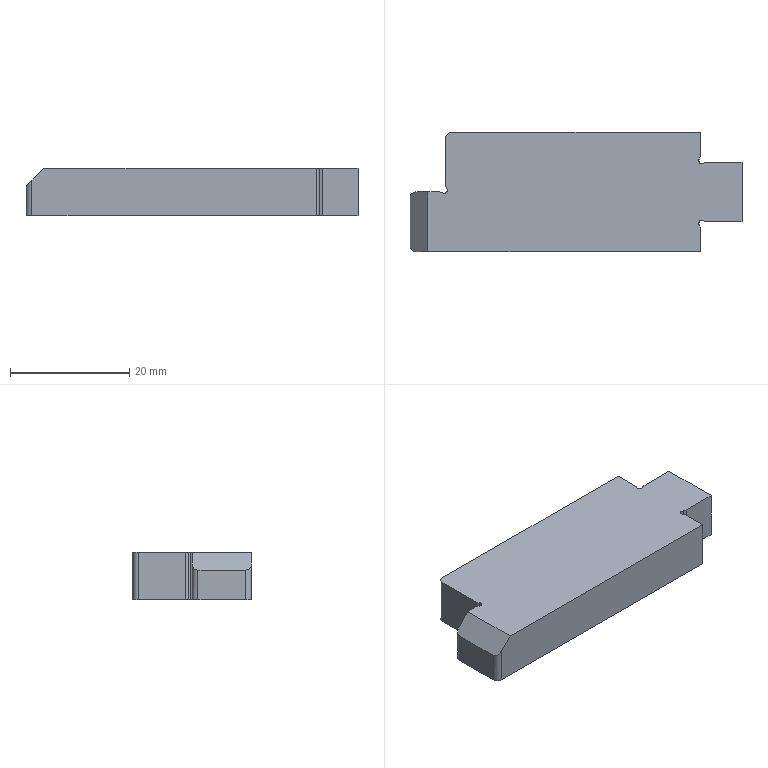Part | SolidWorks | features Chamfer 1, Fillet 1, FlatPattern 1, ICE 1, SMBaseFlange 1, SheetMetal 1 | 1 solid | 26 faces | box 55.7 x 20 x 8 mm | volume 7815 mm3 | cylinder 13 | plane 13 | commonest cylinder face diameters 2 x9 1 x4
STEP:
#1=CARTESIAN_POINT('',(1461.75,307.95,-8.));
#2=VERTEX_POINT('',#1);
#3=CARTESIAN_POINT('',(1461.667,308.226,-8.));
#4=VERTEX_POINT('',#3);
#5=CARTESIAN_POINT('',(1461.25,307.95,-8.));
#6=DIRECTION('',(0.,0.,1.));
#7=DIRECTION('',(1.,0.,0.));
#8=AXIS2_PLACEMENT_3D('',#5,#6,#7);
#9=CIRCLE('',#8,0.5);
#10=EDGE_CURVE('',#2,#4,#9,.T.);
#11=ORIENTED_EDGE('',*,*,#10,.F.);
#12=CARTESIAN_POINT('',(1461.75,307.95,0.));
#13=VERTEX_POINT('',#12);
#14=CARTESIAN_POINT('',(1461.75,307.95,-8.));
#15=DIRECTION('',(0.,0.,1.));
#16=VECTOR('',#15,1000.);
#17=LINE('',#14,#16);
#18=EDGE_CURVE('',#2,#13,#17,.T.);
#19=ORIENTED_EDGE('',*,*,#18,.T.);
#20=CARTESIAN_POINT('',(1461.667,308.226,0.));
#21=VERTEX_POINT('',#20);
#22=CARTESIAN_POINT('',(1461.25,307.95,0.));
#23=DIRECTION('',(0.,0.,1.));
#24=DIRECTION('',(1.,0.,0.));
#25=AXIS2_PLACEMENT_3D('',#22,#23,#24);
#26=CIRCLE('',#25,0.5);
#27=EDGE_CURVE('',#13,#21,#26,.T.);
#28=ORIENTED_EDGE('',*,*,#27,.T.);
#29=CARTESIAN_POINT('',(1461.667,308.226,-8.));
#30=DIRECTION('',(0.,0.,-1.));
#31=VECTOR('',#30,1000.);
#32=LINE('',#29,#31);
#33=EDGE_CURVE('',#21,#4,#32,.T.);
#34=ORIENTED_EDGE('',*,*,#33,.T.);
#35=EDGE_LOOP('',(#11,#19,#28,#34));
#36=FACE_OUTER_BOUND('',#35,.T.);
#37=CARTESIAN_POINT('',(1461.25,307.95,-8.));
#38=DIRECTION('',(0.,0.,1.));
#39=DIRECTION('',(1.,0.,0.));
#40=AXIS2_PLACEMENT_3D('',#37,#38,#39);
#41=CYLINDRICAL_SURFACE('',#40,0.5);
#42=ADVANCED_FACE('',(#36),#41,.F.);
#43=CARTESIAN_POINT('',(1456.5,307.7,-8.));
#44=VERTEX_POINT('',#43);
#45=CARTESIAN_POINT('',(1456.5,307.7,-2.));
#46=VERTEX_POINT('',#45);
#47=CARTESIAN_POINT('',(1456.5,307.7,-8.));
#48=DIRECTION('',(0.,0.,1.));
#49=VECTOR('',#48,1000.);
#50=LINE('',#47,#49);
#51=EDGE_CURVE('',#44,#46,#50,.T.);
#52=ORIENTED_EDGE('',*,*,#51,.T.);
#53=CARTESIAN_POINT('',(1458.5,307.7,0.));
#54=VERTEX_POINT('',#53);
#55=CARTESIAN_POINT('',(1456.,307.7,-2.5));
#56=DIRECTION('',(0.7071,0.,0.7071));
#57=VECTOR('',#56,1000.);
#58=LINE('',#55,#57);
#59=EDGE_CURVE('',#46,#54,#58,.T.);
#60=ORIENTED_EDGE('',*,*,#59,.T.);
#61=CARTESIAN_POINT('',(1460.421,307.7,0.));
#62=VERTEX_POINT('',#61);
#63=CARTESIAN_POINT('',(1461.5,307.7,0.));
#64=DIRECTION('',(-1.,0.,0.));
#65=VECTOR('',#64,1000.);
#66=LINE('',#63,#65);
#67=EDGE_CURVE('',#62,#54,#66,.T.);
#68=ORIENTED_EDGE('',*,*,#67,.F.);
#69=CARTESIAN_POINT('',(1460.421,307.7,-8.));
#70=VERTEX_POINT('',#69);
#71=CARTESIAN_POINT('',(1460.421,307.7,-8.));
#72=DIRECTION('',(0.,0.,-1.));
#73=VECTOR('',#72,1000.);
#74=LINE('',#71,#73);
#75=EDGE_CURVE('',#62,#70,#74,.T.);
#76=ORIENTED_EDGE('',*,*,#75,.T.);
#77=CARTESIAN_POINT('',(1461.5,307.7,-8.));
#78=DIRECTION('',(-1.,0.,0.));
#79=VECTOR('',#78,1000.);
#80=LINE('',#77,#79);
#81=EDGE_CURVE('',#70,#44,#80,.T.);
#82=ORIENTED_EDGE('',*,*,#81,.T.);
#83=EDGE_LOOP('',(#52,#60,#68,#76,#82));
#84=FACE_OUTER_BOUND('',#83,.T.);
#85=CARTESIAN_POINT('',(1461.5,307.7,-8.));
#86=DIRECTION('',(0.,1.,0.));
#87=DIRECTION('',(0.,0.,1.));
#88=AXIS2_PLACEMENT_3D('',#85,#86,#87);
#89=PLANE('',#88);
#90=ADVANCED_FACE('',(#84),#89,.T.);
#91=CARTESIAN_POINT('',(1461.5,316.7,0.));
#92=VERTEX_POINT('',#91);
#93=CARTESIAN_POINT('',(1461.5,308.779,0.));
#94=VERTEX_POINT('',#93);
#95=CARTESIAN_POINT('',(1461.5,317.7,0.));
#96=DIRECTION('',(0.,-1.,0.));
#97=VECTOR('',#96,1000.);
#98=LINE('',#95,#97);
#99=EDGE_CURVE('',#92,#94,#98,.T.);
#100=ORIENTED_EDGE('',*,*,#99,.F.);
#101=CARTESIAN_POINT('',(1461.5,316.7,-8.));
#102=VERTEX_POINT('',#101);
#103=CARTESIAN_POINT('',(1461.5,316.7,-8.));
#104=DIRECTION('',(0.,0.,-1.));
#105=VECTOR('',#104,1000.);
#106=LINE('',#103,#105);
#107=EDGE_CURVE('',#92,#102,#106,.T.);
#108=ORIENTED_EDGE('',*,*,#107,.T.);
#109=CARTESIAN_POINT('',(1461.5,308.779,-8.));
#110=VERTEX_POINT('',#109);
#111=CARTESIAN_POINT('',(1461.5,317.7,-8.));
#112=DIRECTION('',(0.,-1.,0.));
#113=VECTOR('',#112,1000.);
#114=LINE('',#111,#113);
#115=EDGE_CURVE('',#102,#110,#114,.T.);
#116=ORIENTED_EDGE('',*,*,#115,.T.);
#117=CARTESIAN_POINT('',(1461.5,308.779,-8.));
#118=DIRECTION('',(0.,0.,1.));
#119=VECTOR('',#118,1000.);
#120=LINE('',#117,#119);
#121=EDGE_CURVE('',#110,#94,#120,.T.);
#122=ORIENTED_EDGE('',*,*,#121,.T.);
#123=EDGE_LOOP('',(#100,#108,#116,#122));
#124=FACE_OUTER_BOUND('',#123,.T.);
#125=CARTESIAN_POINT('',(1461.5,317.7,-8.));
#126=DIRECTION('',(-1.,0.,0.));
#127=DIRECTION('',(0.,0.,1.));
#128=AXIS2_PLACEMENT_3D('',#125,#126,#127);
#129=PLANE('',#128);
#130=ADVANCED_FACE('',(#124),#129,.T.);
#131=CARTESIAN_POINT('',(1504.2,313.779,0.));
#132=VERTEX_POINT('',#131);
#133=CARTESIAN_POINT('',(1504.2,317.7,0.));
#134=VERTEX_POINT('',#133);
#135=CARTESIAN_POINT('',(1504.2,312.7,0.));
#136=DIRECTION('',(0.,1.,0.));
#137=VECTOR('',#136,1000.);
#138=LINE('',#135,#137);
#139=EDGE_CURVE('',#132,#134,#138,.T.);
#140=ORIENTED_EDGE('',*,*,#139,.F.);
#141=CARTESIAN_POINT('',(1504.2,313.779,-8.));
#142=VERTEX_POINT('',#141);
#143=CARTESIAN_POINT('',(1504.2,313.779,-8.));
#144=DIRECTION('',(0.,0.,-1.));
#145=VECTOR('',#144,1000.);
#146=LINE('',#143,#145);
#147=EDGE_CURVE('',#132,#142,#146,.T.);
#148=ORIENTED_EDGE('',*,*,#147,.T.);
#149=CARTESIAN_POINT('',(1504.2,317.7,-8.));
#150=VERTEX_POINT('',#149);
#151=CARTESIAN_POINT('',(1504.2,312.7,-8.));
#152=DIRECTION('',(0.,1.,0.));
#153=VECTOR('',#152,1000.);
#154=LINE('',#151,#153);
#155=EDGE_CURVE('',#142,#150,#154,.T.);
#156=ORIENTED_EDGE('',*,*,#155,.T.);
#157=CARTESIAN_POINT('',(1504.2,317.7,-8.));
#158=DIRECTION('',(0.,0.,1.));
#159=VECTOR('',#158,1000.);
#160=LINE('',#157,#159);
#161=EDGE_CURVE('',#150,#134,#160,.T.);
#162=ORIENTED_EDGE('',*,*,#161,.T.);
#163=EDGE_LOOP('',(#140,#148,#156,#162));
#164=FACE_OUTER_BOUND('',#163,.T.);
#165=CARTESIAN_POINT('',(1504.2,312.7,-8.));
#166=DIRECTION('',(1.,0.,0.));
#167=DIRECTION('',(0.,0.,-1.));
#168=AXIS2_PLACEMENT_3D('',#165,#166,#167);
#169=PLANE('',#168);
#170=ADVANCED_FACE('',(#164),#169,.T.);
#171=CARTESIAN_POINT('',(1511.2,312.7,-8.));
#172=VERTEX_POINT('',#171);
#173=CARTESIAN_POINT('',(1505.279,312.7,-8.));
#174=VERTEX_POINT('',#173);
#175=CARTESIAN_POINT('',(1511.2,312.7,-8.));
#176=DIRECTION('',(-1.,0.,0.));
#177=VECTOR('',#176,1000.);
#178=LINE('',#175,#177);
#179=EDGE_CURVE('',#172,#174,#178,.T.);
#180=ORIENTED_EDGE('',*,*,#179,.T.);
#181=CARTESIAN_POINT('',(1505.279,312.7,0.));
#182=VERTEX_POINT('',#181);
#183=CARTESIAN_POINT('',(1505.279,312.7,-8.));
#184=DIRECTION('',(0.,0.,1.));
#185=VECTOR('',#184,1000.);
#186=LINE('',#183,#185);
#187=EDGE_CURVE('',#174,#182,#186,.T.);
#188=ORIENTED_EDGE('',*,*,#187,.T.);
#189=CARTESIAN_POINT('',(1511.2,312.7,0.));
#190=VERTEX_POINT('',#189);
#191=CARTESIAN_POINT('',(1511.2,312.7,0.));
#192=DIRECTION('',(-1.,0.,0.));
#193=VECTOR('',#192,1000.);
#194=LINE('',#191,#193);
#195=EDGE_CURVE('',#190,#182,#194,.T.);
#196=ORIENTED_EDGE('',*,*,#195,.F.);
#197=CARTESIAN_POINT('',(1511.2,312.7,-8.));
#198=DIRECTION('',(0.,0.,1.));
#199=VECTOR('',#198,1000.);
#200=LINE('',#197,#199);
#201=EDGE_CURVE('',#172,#190,#200,.T.);
#202=ORIENTED_EDGE('',*,*,#201,.F.);
#203=EDGE_LOOP('',(#180,#188,#196,#202));
#204=FACE_OUTER_BOUND('',#203,.T.);
#205=CARTESIAN_POINT('',(1511.2,312.7,-8.));
#206=DIRECTION('',(0.,1.,0.));
#207=DIRECTION('',(0.,0.,1.));
#208=AXIS2_PLACEMENT_3D('',#205,#206,#207);
#209=PLANE('',#208);
#210=ADVANCED_FACE('',(#204),#209,.T.);
#211=CARTESIAN_POINT('',(1505.279,302.7,0.));
#212=VERTEX_POINT('',#211);
#213=CARTESIAN_POINT('',(1511.2,302.7,0.));
#214=VERTEX_POINT('',#213);
#215=CARTESIAN_POINT('',(1504.2,302.7,0.));
#216=DIRECTION('',(1.,0.,0.));
#217=VECTOR('',#216,1000.);
#218=LINE('',#215,#217);
#219=EDGE_CURVE('',#212,#214,#218,.T.);
#220=ORIENTED_EDGE('',*,*,#219,.F.);
#221=CARTESIAN_POINT('',(1505.279,302.7,-8.));
#222=VERTEX_POINT('',#221);
#223=CARTESIAN_POINT('',(1505.279,302.7,-8.));
#224=DIRECTION('',(0.,0.,-1.));
#225=VECTOR('',#224,1000.);
#226=LINE('',#223,#225);
#227=EDGE_CURVE('',#212,#222,#226,.T.);
#228=ORIENTED_EDGE('',*,*,#227,.T.);
#229=CARTESIAN_POINT('',(1511.2,302.7,-8.));
#230=VERTEX_POINT('',#229);
#231=CARTESIAN_POINT('',(1504.2,302.7,-8.));
#232=DIRECTION('',(1.,0.,0.));
#233=VECTOR('',#232,1000.);
#234=LINE('',#231,#233);
#235=EDGE_CURVE('',#222,#230,#234,.T.);
#236=ORIENTED_EDGE('',*,*,#235,.T.);
#237=CARTESIAN_POINT('',(1511.2,302.7,-8.));
#238=DIRECTION('',(0.,0.,1.));
#239=VECTOR('',#238,1000.);
#240=LINE('',#237,#239);
#241=EDGE_CURVE('',#230,#214,#240,.T.);
#242=ORIENTED_EDGE('',*,*,#241,.T.);
#243=EDGE_LOOP('',(#220,#228,#236,#242));
#244=FACE_OUTER_BOUND('',#243,.T.);
#245=CARTESIAN_POINT('',(1504.2,302.7,-8.));
#246=DIRECTION('',(0.,-1.,0.));
#247=DIRECTION('',(0.,0.,-1.));
#248=AXIS2_PLACEMENT_3D('',#245,#246,#247);
#249=PLANE('',#248);
#250=ADVANCED_FACE('',(#244),#249,.T.);
#251=CARTESIAN_POINT('',(1504.2,297.7,-8.));
#252=VERTEX_POINT('',#251);
#253=CARTESIAN_POINT('',(1504.2,301.621,-8.));
#254=VERTEX_POINT('',#253);
#255=CARTESIAN_POINT('',(1504.2,297.7,-8.));
#256=DIRECTION('',(0.,1.,0.));
#257=VECTOR('',#256,1000.);
#258=LINE('',#255,#257);
#259=EDGE_CURVE('',#252,#254,#258,.T.);
#260=ORIENTED_EDGE('',*,*,#259,.T.);
#261=CARTESIAN_POINT('',(1504.2,301.621,0.));
#262=VERTEX_POINT('',#261);
#263=CARTESIAN_POINT('',(1504.2,301.621,-8.));
#264=DIRECTION('',(0.,0.,1.));
#265=VECTOR('',#264,1000.);
#266=LINE('',#263,#265);
#267=EDGE_CURVE('',#254,#262,#266,.T.);
#268=ORIENTED_EDGE('',*,*,#267,.T.);
#269=CARTESIAN_POINT('',(1504.2,297.7,0.));
#270=VERTEX_POINT('',#269);
#271=CARTESIAN_POINT('',(1504.2,297.7,0.));
#272=DIRECTION('',(0.,1.,0.));
#273=VECTOR('',#272,1000.);
#274=LINE('',#271,#273);
#275=EDGE_CURVE('',#270,#262,#274,.T.);
#276=ORIENTED_EDGE('',*,*,#275,.F.);
#277=CARTESIAN_POINT('',(1504.2,297.7,-8.));
#278=DIRECTION('',(0.,0.,1.));
#279=VECTOR('',#278,1000.);
#280=LINE('',#277,#279);
#281=EDGE_CURVE('',#252,#270,#280,.T.);
#282=ORIENTED_EDGE('',*,*,#281,.F.);
#283=EDGE_LOOP('',(#260,#268,#276,#282));
#284=FACE_OUTER_BOUND('',#283,.T.);
#285=CARTESIAN_POINT('',(1504.2,297.7,-8.));
#286=DIRECTION('',(1.,0.,0.));
#287=DIRECTION('',(0.,0.,-1.));
#288=AXIS2_PLACEMENT_3D('',#285,#286,#287);
#289=PLANE('',#288);
#290=ADVANCED_FACE('',(#284),#289,.T.);
#291=CARTESIAN_POINT('',(1455.5,306.7,-8.));
#292=VERTEX_POINT('',#291);
#293=CARTESIAN_POINT('',(1455.5,298.7,-8.));
#294=VERTEX_POINT('',#293);
#295=CARTESIAN_POINT('',(1455.5,307.7,-8.));
#296=DIRECTION('',(0.,-1.,0.));
#297=VECTOR('',#296,1000.);
#298=LINE('',#295,#297);
#299=EDGE_CURVE('',#292,#294,#298,.T.);
#300=ORIENTED_EDGE('',*,*,#299,.F.);
#301=CARTESIAN_POINT('',(1456.5,306.7,-8.));
#302=DIRECTION('',(0.,0.,-1.));
#303=DIRECTION('',(1.,0.,0.));
#304=AXIS2_PLACEMENT_3D('',#301,#302,#303);
#305=CIRCLE('',#304,1.);
#306=EDGE_CURVE('',#292,#44,#305,.T.);
#307=ORIENTED_EDGE('',*,*,#306,.T.);
#308=ORIENTED_EDGE('',*,*,#81,.F.);
#309=CARTESIAN_POINT('',(1460.974,307.533,-8.));
#310=VERTEX_POINT('',#309);
#311=CARTESIAN_POINT('',(1460.421,306.7,-8.));
#312=DIRECTION('',(0.,0.,-1.));
#313=DIRECTION('',(1.,0.,0.));
#314=AXIS2_PLACEMENT_3D('',#311,#312,#313);
#315=CIRCLE('',#314,1.);
#316=EDGE_CURVE('',#70,#310,#315,.T.);
#317=ORIENTED_EDGE('',*,*,#316,.T.);
#318=CARTESIAN_POINT('',(1461.25,307.95,-8.));
#319=DIRECTION('',(0.,0.,1.));
#320=DIRECTION('',(1.,0.,0.));
#321=AXIS2_PLACEMENT_3D('',#318,#319,#320);
#322=CIRCLE('',#321,0.5);
#323=EDGE_CURVE('',#310,#2,#322,.T.);
#324=ORIENTED_EDGE('',*,*,#323,.T.);
#325=ORIENTED_EDGE('',*,*,#10,.T.);
#326=CARTESIAN_POINT('',(1462.5,308.779,-8.));
#327=DIRECTION('',(0.,0.,-1.));
#328=DIRECTION('',(1.,0.,0.));
#329=AXIS2_PLACEMENT_3D('',#326,#327,#328);
#330=CIRCLE('',#329,1.);
#331=EDGE_CURVE('',#4,#110,#330,.T.);
#332=ORIENTED_EDGE('',*,*,#331,.T.);
#333=ORIENTED_EDGE('',*,*,#115,.F.);
#334=CARTESIAN_POINT('',(1462.5,317.7,-8.));
#335=VERTEX_POINT('',#334);
#336=CARTESIAN_POINT('',(1462.5,316.7,-8.));
#337=DIRECTION('',(0.,0.,-1.));
#338=DIRECTION('',(1.,0.,0.));
#339=AXIS2_PLACEMENT_3D('',#336,#337,#338);
#340=CIRCLE('',#339,1.);
#341=EDGE_CURVE('',#102,#335,#340,.T.);
#342=ORIENTED_EDGE('',*,*,#341,.T.);
#343=CARTESIAN_POINT('',(1504.2,317.7,-8.));
#344=DIRECTION('',(-1.,0.,0.));
#345=VECTOR('',#344,1000.);
#346=LINE('',#343,#345);
#347=EDGE_CURVE('',#150,#335,#346,.T.);
#348=ORIENTED_EDGE('',*,*,#347,.F.);
#349=ORIENTED_EDGE('',*,*,#155,.F.);
#350=CARTESIAN_POINT('',(1504.033,313.226,-8.));
#351=VERTEX_POINT('',#350);
#352=CARTESIAN_POINT('',(1503.2,313.779,-8.));
#353=DIRECTION('',(0.,0.,-1.));
#354=DIRECTION('',(1.,0.,0.));
#355=AXIS2_PLACEMENT_3D('',#352,#353,#354);
#356=CIRCLE('',#355,1.);
#357=EDGE_CURVE('',#142,#351,#356,.T.);
#358=ORIENTED_EDGE('',*,*,#357,.T.);
#359=CARTESIAN_POINT('',(1504.726,312.533,-8.));
#360=VERTEX_POINT('',#359);
#361=CARTESIAN_POINT('',(1504.45,312.95,-8.));
#362=DIRECTION('',(0.,0.,1.));
#363=DIRECTION('',(1.,0.,0.));
#364=AXIS2_PLACEMENT_3D('',#361,#362,#363);
#365=CIRCLE('',#364,0.5);
#366=EDGE_CURVE('',#351,#360,#365,.T.);
#367=ORIENTED_EDGE('',*,*,#366,.T.);
#368=CARTESIAN_POINT('',(1505.279,311.7,-8.));
#369=DIRECTION('',(0.,0.,-1.));
#370=DIRECTION('',(1.,0.,0.));
#371=AXIS2_PLACEMENT_3D('',#368,#369,#370);
#372=CIRCLE('',#371,1.);
#373=EDGE_CURVE('',#360,#174,#372,.T.);
#374=ORIENTED_EDGE('',*,*,#373,.T.);
#375=ORIENTED_EDGE('',*,*,#179,.F.);
#376=CARTESIAN_POINT('',(1511.2,302.7,-8.));
#377=DIRECTION('',(0.,1.,0.));
#378=VECTOR('',#377,1000.);
#379=LINE('',#376,#378);
#380=EDGE_CURVE('',#230,#172,#379,.T.);
#381=ORIENTED_EDGE('',*,*,#380,.F.);
#382=ORIENTED_EDGE('',*,*,#235,.F.);
#383=CARTESIAN_POINT('',(1504.726,302.867,-8.));
#384=VERTEX_POINT('',#383);
#385=CARTESIAN_POINT('',(1505.279,303.7,-8.));
#386=DIRECTION('',(0.,0.,-1.));
#387=DIRECTION('',(1.,0.,0.));
#388=AXIS2_PLACEMENT_3D('',#385,#386,#387);
#389=CIRCLE('',#388,1.);
#390=EDGE_CURVE('',#222,#384,#389,.T.);
#391=ORIENTED_EDGE('',*,*,#390,.T.);
#392=CARTESIAN_POINT('',(1504.033,302.174,-8.));
#393=VERTEX_POINT('',#392);
#394=CARTESIAN_POINT('',(1504.45,302.45,-8.));
#395=DIRECTION('',(0.,0.,1.));
#396=DIRECTION('',(1.,0.,0.));
#397=AXIS2_PLACEMENT_3D('',#394,#395,#396);
#398=CIRCLE('',#397,0.5);
#399=EDGE_CURVE('',#384,#393,#398,.T.);
#400=ORIENTED_EDGE('',*,*,#399,.T.);
#401=CARTESIAN_POINT('',(1503.2,301.621,-8.));
#402=DIRECTION('',(0.,0.,-1.));
#403=DIRECTION('',(1.,0.,0.));
#404=AXIS2_PLACEMENT_3D('',#401,#402,#403);
#405=CIRCLE('',#404,1.);
#406=EDGE_CURVE('',#393,#254,#405,.T.);
#407=ORIENTED_EDGE('',*,*,#406,.T.);
#408=ORIENTED_EDGE('',*,*,#259,.F.);
#409=CARTESIAN_POINT('',(1456.5,297.7,-8.));
#410=VERTEX_POINT('',#409);
#411=CARTESIAN_POINT('',(1455.5,297.7,-8.));
#412=DIRECTION('',(1.,0.,0.));
#413=VECTOR('',#412,1000.);
#414=LINE('',#411,#413);
#415=EDGE_CURVE('',#410,#252,#414,.T.);
#416=ORIENTED_EDGE('',*,*,#415,.F.);
#417=CARTESIAN_POINT('',(1456.5,298.7,-8.));
#418=DIRECTION('',(0.,0.,-1.));
#419=DIRECTION('',(1.,0.,0.));
#420=AXIS2_PLACEMENT_3D('',#417,#418,#419);
#421=CIRCLE('',#420,1.);
#422=EDGE_CURVE('',#410,#294,#421,.T.);
#423=ORIENTED_EDGE('',*,*,#422,.T.);
#424=EDGE_LOOP('',(#300,#307,#308,#317,#324,#325,#332,#333,#342,#348,#349,#358,#367,#374,#375,#381,#382,#391,#400,#407,#408,#416,#423));
#425=FACE_OUTER_BOUND('',#424,.T.);
#426=CARTESIAN_POINT('',(0.,0.,-8.));
#427=DIRECTION('',(0.,0.,1.));
#428=DIRECTION('',(1.,0.,0.));
#429=AXIS2_PLACEMENT_3D('',#426,#427,#428);
#430=PLANE('',#429);
#431=ADVANCED_FACE('',(#425),#430,.F.);
#432=ORIENTED_EDGE('',*,*,#67,.T.);
#433=CARTESIAN_POINT('',(1458.5,297.7,0.));
#434=VERTEX_POINT('',#433);
#435=CARTESIAN_POINT('',(1458.5,0.,0.));
#436=DIRECTION('',(0.,-1.,0.));
#437=VECTOR('',#436,1000.);
#438=LINE('',#435,#437);
#439=EDGE_CURVE('',#54,#434,#438,.T.);
#440=ORIENTED_EDGE('',*,*,#439,.T.);
#441=CARTESIAN_POINT('',(1455.5,297.7,0.));
#442=DIRECTION('',(1.,0.,0.));
#443=VECTOR('',#442,1000.);
#444=LINE('',#441,#443);
#445=EDGE_CURVE('',#434,#270,#444,.T.);
#446=ORIENTED_EDGE('',*,*,#445,.T.);
#447=ORIENTED_EDGE('',*,*,#275,.T.);
#448=CARTESIAN_POINT('',(1504.033,302.174,0.));
#449=VERTEX_POINT('',#448);
#450=CARTESIAN_POINT('',(1503.2,301.621,0.));
#451=DIRECTION('',(0.,0.,1.));
#452=DIRECTION('',(1.,0.,0.));
#453=AXIS2_PLACEMENT_3D('',#450,#451,#452);
#454=CIRCLE('',#453,1.);
#455=EDGE_CURVE('',#262,#449,#454,.T.);
#456=ORIENTED_EDGE('',*,*,#455,.T.);
#457=CARTESIAN_POINT('',(1504.726,302.867,0.));
#458=VERTEX_POINT('',#457);
#459=CARTESIAN_POINT('',(1504.45,302.45,0.));
#460=DIRECTION('',(0.,0.,1.));
#461=DIRECTION('',(1.,0.,0.));
#462=AXIS2_PLACEMENT_3D('',#459,#460,#461);
#463=CIRCLE('',#462,0.5);
#464=EDGE_CURVE('',#458,#449,#463,.T.);
#465=ORIENTED_EDGE('',*,*,#464,.F.);
#466=CARTESIAN_POINT('',(1505.279,303.7,0.));
#467=DIRECTION('',(0.,0.,1.));
#468=DIRECTION('',(1.,0.,0.));
#469=AXIS2_PLACEMENT_3D('',#466,#467,#468);
#470=CIRCLE('',#469,1.);
#471=EDGE_CURVE('',#458,#212,#470,.T.);
#472=ORIENTED_EDGE('',*,*,#471,.T.);
#473=ORIENTED_EDGE('',*,*,#219,.T.);
#474=CARTESIAN_POINT('',(1511.2,302.7,0.));
#475=DIRECTION('',(0.,1.,0.));
#476=VECTOR('',#475,1000.);
#477=LINE('',#474,#476);
#478=EDGE_CURVE('',#214,#190,#477,.T.);
#479=ORIENTED_EDGE('',*,*,#478,.T.);
#480=ORIENTED_EDGE('',*,*,#195,.T.);
#481=CARTESIAN_POINT('',(1504.726,312.533,0.));
#482=VERTEX_POINT('',#481);
#483=CARTESIAN_POINT('',(1505.279,311.7,0.));
#484=DIRECTION('',(0.,0.,1.));
#485=DIRECTION('',(1.,0.,0.));
#486=AXIS2_PLACEMENT_3D('',#483,#484,#485);
#487=CIRCLE('',#486,1.);
#488=EDGE_CURVE('',#182,#482,#487,.T.);
#489=ORIENTED_EDGE('',*,*,#488,.T.);
#490=CARTESIAN_POINT('',(1504.033,313.226,0.));
#491=VERTEX_POINT('',#490);
#492=CARTESIAN_POINT('',(1504.45,312.95,0.));
#493=DIRECTION('',(0.,0.,1.));
#494=DIRECTION('',(1.,0.,0.));
#495=AXIS2_PLACEMENT_3D('',#492,#493,#494);
#496=CIRCLE('',#495,0.5);
#497=EDGE_CURVE('',#491,#482,#496,.T.);
#498=ORIENTED_EDGE('',*,*,#497,.F.);
#499=CARTESIAN_POINT('',(1503.2,313.779,0.));
#500=DIRECTION('',(0.,0.,1.));
#501=DIRECTION('',(1.,0.,0.));
#502=AXIS2_PLACEMENT_3D('',#499,#500,#501);
#503=CIRCLE('',#502,1.);
#504=EDGE_CURVE('',#491,#132,#503,.T.);
#505=ORIENTED_EDGE('',*,*,#504,.T.);
#506=ORIENTED_EDGE('',*,*,#139,.T.);
#507=CARTESIAN_POINT('',(1462.5,317.7,0.));
#508=VERTEX_POINT('',#507);
#509=CARTESIAN_POINT('',(1504.2,317.7,0.));
#510=DIRECTION('',(-1.,0.,0.));
#511=VECTOR('',#510,1000.);
#512=LINE('',#509,#511);
#513=EDGE_CURVE('',#134,#508,#512,.T.);
#514=ORIENTED_EDGE('',*,*,#513,.T.);
#515=CARTESIAN_POINT('',(1462.5,316.7,0.));
#516=DIRECTION('',(0.,0.,1.));
#517=DIRECTION('',(1.,0.,0.));
#518=AXIS2_PLACEMENT_3D('',#515,#516,#517);
#519=CIRCLE('',#518,1.);
#520=EDGE_CURVE('',#508,#92,#519,.T.);
#521=ORIENTED_EDGE('',*,*,#520,.T.);
#522=ORIENTED_EDGE('',*,*,#99,.T.);
#523=CARTESIAN_POINT('',(1462.5,308.779,0.));
#524=DIRECTION('',(0.,0.,1.));
#525=DIRECTION('',(1.,0.,0.));
#526=AXIS2_PLACEMENT_3D('',#523,#524,#525);
#527=CIRCLE('',#526,1.);
#528=EDGE_CURVE('',#94,#21,#527,.T.);
#529=ORIENTED_EDGE('',*,*,#528,.T.);
#530=ORIENTED_EDGE('',*,*,#27,.F.);
#531=CARTESIAN_POINT('',(1460.974,307.533,0.));
#532=VERTEX_POINT('',#531);
#533=CARTESIAN_POINT('',(1461.25,307.95,0.));
#534=DIRECTION('',(0.,0.,1.));
#535=DIRECTION('',(1.,0.,0.));
#536=AXIS2_PLACEMENT_3D('',#533,#534,#535);
#537=CIRCLE('',#536,0.5);
#538=EDGE_CURVE('',#532,#13,#537,.T.);
#539=ORIENTED_EDGE('',*,*,#538,.F.);
#540=CARTESIAN_POINT('',(1460.421,306.7,0.));
#541=DIRECTION('',(0.,0.,1.));
#542=DIRECTION('',(1.,0.,0.));
#543=AXIS2_PLACEMENT_3D('',#540,#541,#542);
#544=CIRCLE('',#543,1.);
#545=EDGE_CURVE('',#532,#62,#544,.T.);
#546=ORIENTED_EDGE('',*,*,#545,.T.);
#547=EDGE_LOOP('',(#432,#440,#446,#447,#456,#465,#472,#473,#479,#480,#489,#498,#505,#506,#514,#521,#522,#529,#530,#539,#546));
#548=FACE_OUTER_BOUND('',#547,.T.);
#549=CARTESIAN_POINT('',(0.,0.,0.));
#550=DIRECTION('',(0.,0.,1.));
#551=DIRECTION('',(1.,0.,0.));
#552=AXIS2_PLACEMENT_3D('',#549,#550,#551);
#553=PLANE('',#552);
#554=ADVANCED_FACE('',(#548),#553,.T.);
#555=ORIENTED_EDGE('',*,*,#347,.T.);
#556=CARTESIAN_POINT('',(1462.5,317.7,-8.));
#557=DIRECTION('',(0.,0.,1.));
#558=VECTOR('',#557,1000.);
#559=LINE('',#556,#558);
#560=EDGE_CURVE('',#335,#508,#559,.T.);
#561=ORIENTED_EDGE('',*,*,#560,.T.);
#562=ORIENTED_EDGE('',*,*,#513,.F.);
#563=ORIENTED_EDGE('',*,*,#161,.F.);
#564=EDGE_LOOP('',(#555,#561,#562,#563));
#565=FACE_OUTER_BOUND('',#564,.T.);
#566=CARTESIAN_POINT('',(1504.2,317.7,-8.));
#567=DIRECTION('',(0.,1.,0.));
#568=DIRECTION('',(0.,0.,1.));
#569=AXIS2_PLACEMENT_3D('',#566,#567,#568);
#570=PLANE('',#569);
#571=ADVANCED_FACE('',(#565),#570,.T.);
#572=ORIENTED_EDGE('',*,*,#478,.F.);
#573=ORIENTED_EDGE('',*,*,#241,.F.);
#574=ORIENTED_EDGE('',*,*,#380,.T.);
#575=ORIENTED_EDGE('',*,*,#201,.T.);
#576=EDGE_LOOP('',(#572,#573,#574,#575));
#577=FACE_OUTER_BOUND('',#576,.T.);
#578=CARTESIAN_POINT('',(1511.2,302.7,-8.));
#579=DIRECTION('',(1.,0.,0.));
#580=DIRECTION('',(0.,0.,-1.));
#581=AXIS2_PLACEMENT_3D('',#578,#579,#580);
#582=PLANE('',#581);
#583=ADVANCED_FACE('',(#577),#582,.T.);
#584=ORIENTED_EDGE('',*,*,#445,.F.);
#585=CARTESIAN_POINT('',(1456.5,297.7,-2.));
#586=VERTEX_POINT('',#585);
#587=CARTESIAN_POINT('',(1453.,297.7,-5.5));
#588=DIRECTION('',(-0.7071,0.,-0.7071));
#589=VECTOR('',#588,1000.);
#590=LINE('',#587,#589);
#591=EDGE_CURVE('',#434,#586,#590,.T.);
#592=ORIENTED_EDGE('',*,*,#591,.T.);
#593=CARTESIAN_POINT('',(1456.5,297.7,-8.));
#594=DIRECTION('',(0.,0.,-1.));
#595=VECTOR('',#594,1000.);
#596=LINE('',#593,#595);
#597=EDGE_CURVE('',#586,#410,#596,.T.);
#598=ORIENTED_EDGE('',*,*,#597,.T.);
#599=ORIENTED_EDGE('',*,*,#415,.T.);
#600=ORIENTED_EDGE('',*,*,#281,.T.);
#601=EDGE_LOOP('',(#584,#592,#598,#599,#600));
#602=FACE_OUTER_BOUND('',#601,.T.);
#603=CARTESIAN_POINT('',(1455.5,297.7,-8.));
#604=DIRECTION('',(0.,-1.,0.));
#605=DIRECTION('',(0.,0.,-1.));
#606=AXIS2_PLACEMENT_3D('',#603,#604,#605);
#607=PLANE('',#606);
#608=ADVANCED_FACE('',(#602),#607,.T.);
#609=CARTESIAN_POINT('',(1455.5,298.7,-3.));
#610=VERTEX_POINT('',#609);
#611=CARTESIAN_POINT('',(1455.5,298.7,-8.));
#612=DIRECTION('',(0.,0.,1.));
#613=VECTOR('',#612,1000.);
#614=LINE('',#611,#613);
#615=EDGE_CURVE('',#294,#610,#614,.T.);
#616=ORIENTED_EDGE('',*,*,#615,.T.);
#617=CARTESIAN_POINT('',(1455.5,306.7,-3.));
#618=VERTEX_POINT('',#617);
#619=CARTESIAN_POINT('',(1455.5,307.7,-3.));
#620=DIRECTION('',(0.,1.,0.));
#621=VECTOR('',#620,1000.);
#622=LINE('',#619,#621);
#623=EDGE_CURVE('',#610,#618,#622,.T.);
#624=ORIENTED_EDGE('',*,*,#623,.T.);
#625=CARTESIAN_POINT('',(1455.5,306.7,-8.));
#626=DIRECTION('',(0.,0.,-1.));
#627=VECTOR('',#626,1000.);
#628=LINE('',#625,#627);
#629=EDGE_CURVE('',#618,#292,#628,.T.);
#630=ORIENTED_EDGE('',*,*,#629,.T.);
#631=ORIENTED_EDGE('',*,*,#299,.T.);
#632=EDGE_LOOP('',(#616,#624,#630,#631));
#633=FACE_OUTER_BOUND('',#632,.T.);
#634=CARTESIAN_POINT('',(1455.5,307.7,-8.));
#635=DIRECTION('',(-1.,0.,0.));
#636=DIRECTION('',(0.,0.,1.));
#637=AXIS2_PLACEMENT_3D('',#634,#635,#636);
#638=PLANE('',#637);
#639=ADVANCED_FACE('',(#633),#638,.T.);
#640=ORIENTED_EDGE('',*,*,#497,.T.);
#641=CARTESIAN_POINT('',(1504.726,312.533,-8.));
#642=DIRECTION('',(0.,0.,-1.));
#643=VECTOR('',#642,1000.);
#644=LINE('',#641,#643);
#645=EDGE_CURVE('',#482,#360,#644,.T.);
#646=ORIENTED_EDGE('',*,*,#645,.T.);
#647=ORIENTED_EDGE('',*,*,#366,.F.);
#648=CARTESIAN_POINT('',(1504.033,313.226,-8.));
#649=DIRECTION('',(0.,0.,1.));
#650=VECTOR('',#649,1000.);
#651=LINE('',#648,#650);
#652=EDGE_CURVE('',#351,#491,#651,.T.);
#653=ORIENTED_EDGE('',*,*,#652,.T.);
#654=EDGE_LOOP('',(#640,#646,#647,#653));
#655=FACE_OUTER_BOUND('',#654,.T.);
#656=CARTESIAN_POINT('',(1504.45,312.95,-8.));
#657=DIRECTION('',(0.,0.,1.));
#658=DIRECTION('',(1.,0.,0.));
#659=AXIS2_PLACEMENT_3D('',#656,#657,#658);
#660=CYLINDRICAL_SURFACE('',#659,0.5);
#661=ADVANCED_FACE('',(#655),#660,.F.);
#662=ORIENTED_EDGE('',*,*,#18,.F.);
#663=ORIENTED_EDGE('',*,*,#323,.F.);
#664=CARTESIAN_POINT('',(1460.974,307.533,-8.));
#665=DIRECTION('',(0.,0.,1.));
#666=VECTOR('',#665,1000.);
#667=LINE('',#664,#666);
#668=EDGE_CURVE('',#310,#532,#667,.T.);
#669=ORIENTED_EDGE('',*,*,#668,.T.);
#670=ORIENTED_EDGE('',*,*,#538,.T.);
#671=EDGE_LOOP('',(#662,#663,#669,#670));
#672=FACE_OUTER_BOUND('',#671,.T.);
#673=CARTESIAN_POINT('',(1461.25,307.95,-8.));
#674=DIRECTION('',(0.,0.,1.));
#675=DIRECTION('',(1.,0.,0.));
#676=AXIS2_PLACEMENT_3D('',#673,#674,#675);
#677=CYLINDRICAL_SURFACE('',#676,0.5);
#678=ADVANCED_FACE('',(#672),#677,.F.);
#679=ORIENTED_EDGE('',*,*,#399,.F.);
#680=CARTESIAN_POINT('',(1504.726,302.867,-8.));
#681=DIRECTION('',(0.,0.,1.));
#682=VECTOR('',#681,1000.);
#683=LINE('',#680,#682);
#684=EDGE_CURVE('',#384,#458,#683,.T.);
#685=ORIENTED_EDGE('',*,*,#684,.T.);
#686=ORIENTED_EDGE('',*,*,#464,.T.);
#687=CARTESIAN_POINT('',(1504.033,302.174,-8.));
#688=DIRECTION('',(0.,0.,-1.));
#689=VECTOR('',#688,1000.);
#690=LINE('',#687,#689);
#691=EDGE_CURVE('',#449,#393,#690,.T.);
#692=ORIENTED_EDGE('',*,*,#691,.T.);
#693=EDGE_LOOP('',(#679,#685,#686,#692));
#694=FACE_OUTER_BOUND('',#693,.T.);
#695=CARTESIAN_POINT('',(1504.45,302.45,-8.));
#696=DIRECTION('',(0.,0.,1.));
#697=DIRECTION('',(1.,0.,0.));
#698=AXIS2_PLACEMENT_3D('',#695,#696,#697);
#699=CYLINDRICAL_SURFACE('',#698,0.5);
#700=ADVANCED_FACE('',(#694),#699,.F.);
#701=ORIENTED_EDGE('',*,*,#629,.F.);
#702=CARTESIAN_POINT('',(1455.5,306.7,-3.));
#703=CARTESIAN_POINT('',(1455.5,307.286,-3.));
#704=CARTESIAN_POINT('',(1455.914,307.7,-2.586));
#705=CARTESIAN_POINT('',(1456.5,307.7,-2.));
#706=(BOUNDED_CURVE()B_SPLINE_CURVE(3,(#702,#703,#704,#705),.UNSPECIFIED.,.F.,.T.)B_SPLINE_CURVE_WITH_KNOTS((4,4),(3.142,4.712),.UNSPECIFIED.)CURVE()GEOMETRIC_REPRESENTATION_ITEM()RATIONAL_B_SPLINE_CURVE((1.,0.8047,0.8047,1.))REPRESENTATION_ITEM(''));
#707=EDGE_CURVE('',#618,#46,#706,.T.);
#708=ORIENTED_EDGE('',*,*,#707,.T.);
#709=ORIENTED_EDGE('',*,*,#51,.F.);
#710=ORIENTED_EDGE('',*,*,#306,.F.);
#711=EDGE_LOOP('',(#701,#708,#709,#710));
#712=FACE_OUTER_BOUND('',#711,.T.);
#713=CARTESIAN_POINT('',(1456.5,306.7,-8.));
#714=DIRECTION('',(0.,0.,1.));
#715=DIRECTION('',(1.,0.,0.));
#716=AXIS2_PLACEMENT_3D('',#713,#714,#715);
#717=CYLINDRICAL_SURFACE('',#716,1.);
#718=ADVANCED_FACE('',(#712),#717,.T.);
#719=ORIENTED_EDGE('',*,*,#597,.F.);
#720=CARTESIAN_POINT('',(1456.5,297.7,-2.));
#721=CARTESIAN_POINT('',(1455.914,297.7,-2.586));
#722=CARTESIAN_POINT('',(1455.5,298.114,-3.));
#723=CARTESIAN_POINT('',(1455.5,298.7,-3.));
#724=(BOUNDED_CURVE()B_SPLINE_CURVE(3,(#720,#721,#722,#723),.UNSPECIFIED.,.F.,.T.)B_SPLINE_CURVE_WITH_KNOTS((4,4),(1.571,3.142),.UNSPECIFIED.)CURVE()GEOMETRIC_REPRESENTATION_ITEM()RATIONAL_B_SPLINE_CURVE((1.,0.8047,0.8047,1.))REPRESENTATION_ITEM(''));
#725=EDGE_CURVE('',#586,#610,#724,.T.);
#726=ORIENTED_EDGE('',*,*,#725,.T.);
#727=ORIENTED_EDGE('',*,*,#615,.F.);
#728=ORIENTED_EDGE('',*,*,#422,.F.);
#729=EDGE_LOOP('',(#719,#726,#727,#728));
#730=FACE_OUTER_BOUND('',#729,.T.);
#731=CARTESIAN_POINT('',(1456.5,298.7,-8.));
#732=DIRECTION('',(0.,0.,1.));
#733=DIRECTION('',(1.,0.,0.));
#734=AXIS2_PLACEMENT_3D('',#731,#732,#733);
#735=CYLINDRICAL_SURFACE('',#734,1.);
#736=ADVANCED_FACE('',(#730),#735,.T.);
#737=ORIENTED_EDGE('',*,*,#341,.F.);
#738=ORIENTED_EDGE('',*,*,#107,.F.);
#739=ORIENTED_EDGE('',*,*,#520,.F.);
#740=ORIENTED_EDGE('',*,*,#560,.F.);
#741=EDGE_LOOP('',(#737,#738,#739,#740));
#742=FACE_OUTER_BOUND('',#741,.T.);
#743=CARTESIAN_POINT('',(1462.5,316.7,-8.));
#744=DIRECTION('',(0.,0.,1.));
#745=DIRECTION('',(1.,0.,0.));
#746=AXIS2_PLACEMENT_3D('',#743,#744,#745);
#747=CYLINDRICAL_SURFACE('',#746,1.);
#748=ADVANCED_FACE('',(#742),#747,.T.);
#749=ORIENTED_EDGE('',*,*,#373,.F.);
#750=ORIENTED_EDGE('',*,*,#645,.F.);
#751=ORIENTED_EDGE('',*,*,#488,.F.);
#752=ORIENTED_EDGE('',*,*,#187,.F.);
#753=EDGE_LOOP('',(#749,#750,#751,#752));
#754=FACE_OUTER_BOUND('',#753,.T.);
#755=CARTESIAN_POINT('',(1505.279,311.7,-8.));
#756=DIRECTION('',(0.,0.,1.));
#757=DIRECTION('',(1.,0.,0.));
#758=AXIS2_PLACEMENT_3D('',#755,#756,#757);
#759=CYLINDRICAL_SURFACE('',#758,1.);
#760=ADVANCED_FACE('',(#754),#759,.T.);
#761=ORIENTED_EDGE('',*,*,#357,.F.);
#762=ORIENTED_EDGE('',*,*,#147,.F.);
#763=ORIENTED_EDGE('',*,*,#504,.F.);
#764=ORIENTED_EDGE('',*,*,#652,.F.);
#765=EDGE_LOOP('',(#761,#762,#763,#764));
#766=FACE_OUTER_BOUND('',#765,.T.);
#767=CARTESIAN_POINT('',(1503.2,313.779,-8.));
#768=DIRECTION('',(0.,0.,1.));
#769=DIRECTION('',(1.,0.,0.));
#770=AXIS2_PLACEMENT_3D('',#767,#768,#769);
#771=CYLINDRICAL_SURFACE('',#770,1.);
#772=ADVANCED_FACE('',(#766),#771,.T.);
#773=ORIENTED_EDGE('',*,*,#390,.F.);
#774=ORIENTED_EDGE('',*,*,#227,.F.);
#775=ORIENTED_EDGE('',*,*,#471,.F.);
#776=ORIENTED_EDGE('',*,*,#684,.F.);
#777=EDGE_LOOP('',(#773,#774,#775,#776));
#778=FACE_OUTER_BOUND('',#777,.T.);
#779=CARTESIAN_POINT('',(1505.279,303.7,-8.));
#780=DIRECTION('',(0.,0.,1.));
#781=DIRECTION('',(1.,0.,0.));
#782=AXIS2_PLACEMENT_3D('',#779,#780,#781);
#783=CYLINDRICAL_SURFACE('',#782,1.);
#784=ADVANCED_FACE('',(#778),#783,.T.);
#785=ORIENTED_EDGE('',*,*,#406,.F.);
#786=ORIENTED_EDGE('',*,*,#691,.F.);
#787=ORIENTED_EDGE('',*,*,#455,.F.);
#788=ORIENTED_EDGE('',*,*,#267,.F.);
#789=EDGE_LOOP('',(#785,#786,#787,#788));
#790=FACE_OUTER_BOUND('',#789,.T.);
#791=CARTESIAN_POINT('',(1503.2,301.621,-8.));
#792=DIRECTION('',(0.,0.,1.));
#793=DIRECTION('',(1.,0.,0.));
#794=AXIS2_PLACEMENT_3D('',#791,#792,#793);
#795=CYLINDRICAL_SURFACE('',#794,1.);
#796=ADVANCED_FACE('',(#790),#795,.T.);
#797=ORIENTED_EDGE('',*,*,#331,.F.);
#798=ORIENTED_EDGE('',*,*,#33,.F.);
#799=ORIENTED_EDGE('',*,*,#528,.F.);
#800=ORIENTED_EDGE('',*,*,#121,.F.);
#801=EDGE_LOOP('',(#797,#798,#799,#800));
#802=FACE_OUTER_BOUND('',#801,.T.);
#803=CARTESIAN_POINT('',(1462.5,308.779,-8.));
#804=DIRECTION('',(0.,0.,1.));
#805=DIRECTION('',(1.,0.,0.));
#806=AXIS2_PLACEMENT_3D('',#803,#804,#805);
#807=CYLINDRICAL_SURFACE('',#806,1.);
#808=ADVANCED_FACE('',(#802),#807,.T.);
#809=ORIENTED_EDGE('',*,*,#316,.F.);
#810=ORIENTED_EDGE('',*,*,#75,.F.);
#811=ORIENTED_EDGE('',*,*,#545,.F.);
#812=ORIENTED_EDGE('',*,*,#668,.F.);
#813=EDGE_LOOP('',(#809,#810,#811,#812));
#814=FACE_OUTER_BOUND('',#813,.T.);
#815=CARTESIAN_POINT('',(1460.421,306.7,-8.));
#816=DIRECTION('',(0.,0.,1.));
#817=DIRECTION('',(1.,0.,0.));
#818=AXIS2_PLACEMENT_3D('',#815,#816,#817);
#819=CYLINDRICAL_SURFACE('',#818,1.);
#820=ADVANCED_FACE('',(#814),#819,.T.);
#821=ORIENTED_EDGE('',*,*,#707,.F.);
#822=ORIENTED_EDGE('',*,*,#623,.F.);
#823=ORIENTED_EDGE('',*,*,#725,.F.);
#824=ORIENTED_EDGE('',*,*,#591,.F.);
#825=ORIENTED_EDGE('',*,*,#439,.F.);
#826=ORIENTED_EDGE('',*,*,#59,.F.);
#827=EDGE_LOOP('',(#821,#822,#823,#824,#825,#826));
#828=FACE_OUTER_BOUND('',#827,.T.);
#829=CARTESIAN_POINT('',(1458.5,0.,0.));
#830=DIRECTION('',(0.7071,0.,-0.7071));
#831=DIRECTION('',(0.,-1.,0.));
#832=AXIS2_PLACEMENT_3D('',#829,#830,#831);
#833=PLANE('',#832);
#834=ADVANCED_FACE('',(#828),#833,.F.);
#835=CLOSED_SHELL('',(#42,#90,#130,#170,#210,#250,#290,#431,#554,#571,#583,#608,#639,#661,#678,#700,#718,#736,#748,#760,#772,#784,#796,#808,#820,#834));
#836=MANIFOLD_SOLID_BREP('',#835);
#837=CARTESIAN_POINT('',(0.,0.,0.));
#838=DIRECTION('',(0.,0.,1.));
#839=DIRECTION('',(1.,0.,0.));
#840=AXIS2_PLACEMENT_3D('',#837,#838,#839);
#841=(LENGTH_UNIT()NAMED_UNIT(*)SI_UNIT(.MILLI.,.METRE.));
#842=UNCERTAINTY_MEASURE_WITH_UNIT(LENGTH_MEASURE(0.00001),#841,'','');
#843=(NAMED_UNIT(*)PLANE_ANGLE_UNIT()SI_UNIT($,.RADIAN.));
#844=(NAMED_UNIT(*)SI_UNIT($,.STERADIAN.)SOLID_ANGLE_UNIT());
#845=(GEOMETRIC_REPRESENTATION_CONTEXT(3)GLOBAL_UNCERTAINTY_ASSIGNED_CONTEXT((#842))GLOBAL_UNIT_ASSIGNED_CONTEXT((#841,#843,#844))REPRESENTATION_CONTEXT('',''));
#846=ADVANCED_BREP_SHAPE_REPRESENTATION('',(#836,#840),#845);